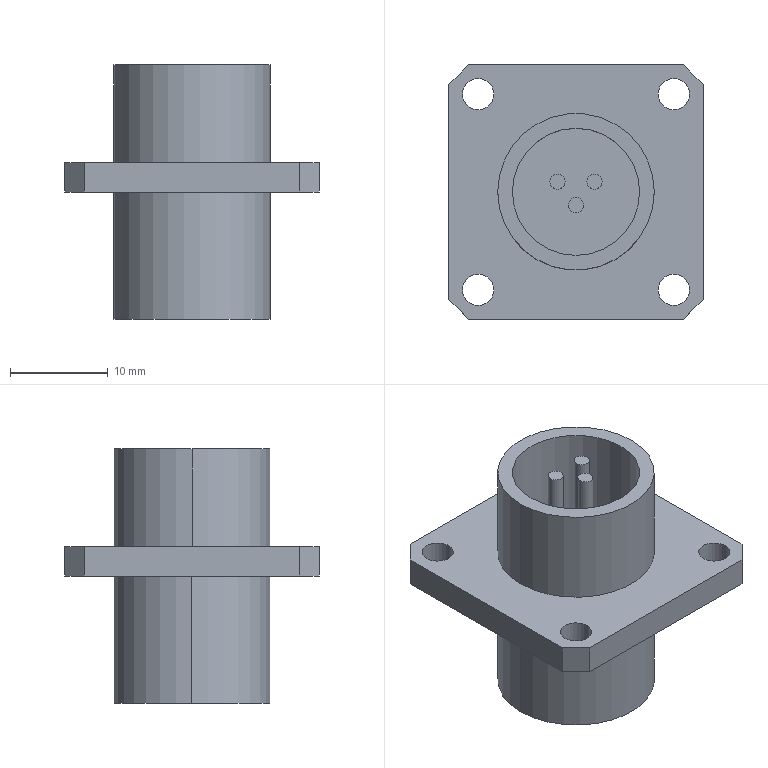Part | STEP file | Aviation plug | 1 solid | 36 faces | box 26 x 26 x 26 mm | volume 5262 mm3 | cylinder 20 | plane 16 | commonest cylinder face diameters 3.2 x8 1.558 x6 16 x4 13 x2